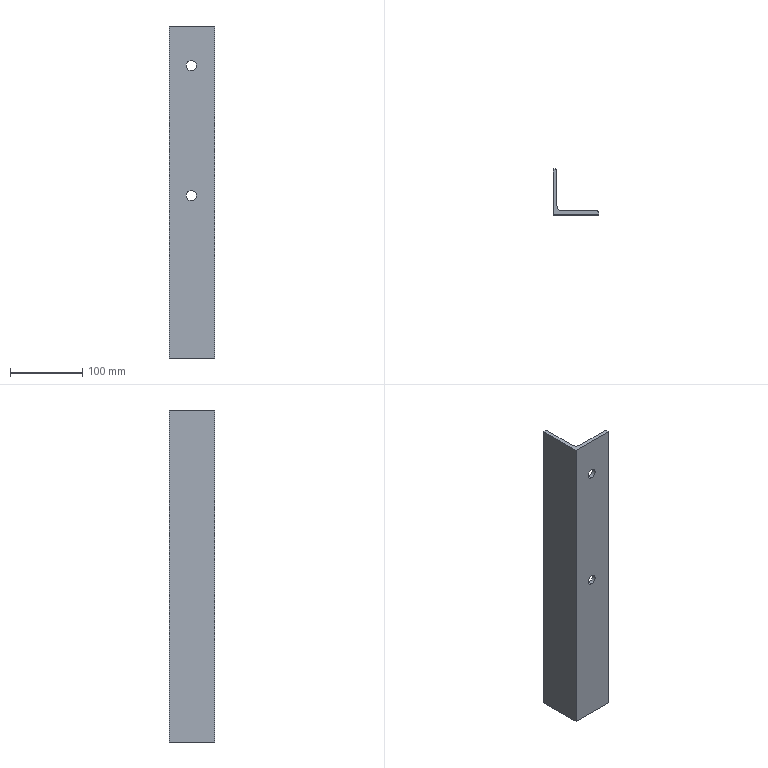Part | NX | features BREP 1 | 1 solid | 15 faces | box 63 x 63 x 460 mm | volume 280553 mm3 | plane 8 | cylinder 7 | commonest cylinder face diameters 14 x5 4.6 x2
STEP:
#1=CARTESIAN_POINT('',(30.5,5.,412.));
#2=VERTEX_POINT('',#1);
#3=CARTESIAN_POINT('',(30.5,5.,398.));
#4=VERTEX_POINT('',#3);
#5=CARTESIAN_POINT('',(30.5,5.,405.));
#6=DIRECTION('',(0.,-1.,0.));
#7=DIRECTION('',(0.,0.,-1.));
#8=AXIS2_PLACEMENT_3D('',#5,#6,#7);
#9=CIRCLE('',#8,7.);
#10=EDGE_CURVE('',#2,#4,#9,.T.);
#11=ORIENTED_EDGE('',*,*,#10,.F.);
#12=CARTESIAN_POINT('',(30.5,0.,412.));
#13=VERTEX_POINT('',#12);
#14=CARTESIAN_POINT('',(30.5,63.,412.));
#15=DIRECTION('',(0.,-1.,0.));
#16=VECTOR('',#15,1000.);
#17=LINE('',#14,#16);
#18=EDGE_CURVE('',#13,#2,#17,.F.);
#19=ORIENTED_EDGE('',*,*,#18,.F.);
#20=CARTESIAN_POINT('',(30.5,0.,398.));
#21=VERTEX_POINT('',#20);
#22=CARTESIAN_POINT('',(30.5,0.,405.));
#23=DIRECTION('',(0.,-1.,0.));
#24=DIRECTION('',(0.,0.,-1.));
#25=AXIS2_PLACEMENT_3D('',#22,#23,#24);
#26=CIRCLE('',#25,7.);
#27=EDGE_CURVE('',#13,#21,#26,.T.);
#28=ORIENTED_EDGE('',*,*,#27,.T.);
#29=CARTESIAN_POINT('',(30.5,63.,398.));
#30=DIRECTION('',(0.,-1.,0.));
#31=VECTOR('',#30,1000.);
#32=LINE('',#29,#31);
#33=EDGE_CURVE('',#21,#4,#32,.F.);
#34=ORIENTED_EDGE('',*,*,#33,.T.);
#35=EDGE_LOOP('',(#11,#19,#28,#34));
#36=FACE_BOUND('',#35,.T.);
#37=CARTESIAN_POINT('',(30.5,63.,405.));
#38=DIRECTION('',(0.,-1.,0.));
#39=DIRECTION('',(0.,0.,1.));
#40=AXIS2_PLACEMENT_3D('',#37,#38,#39);
#41=CYLINDRICAL_SURFACE('',#40,7.);
#42=ADVANCED_FACE('',(#36),#41,.F.);
#43=CARTESIAN_POINT('',(30.5,5.,232.));
#44=VERTEX_POINT('',#43);
#45=CARTESIAN_POINT('',(30.5,5.,218.));
#46=VERTEX_POINT('',#45);
#47=CARTESIAN_POINT('',(30.5,5.,225.));
#48=DIRECTION('',(0.,-1.,0.));
#49=DIRECTION('',(0.,0.,-1.));
#50=AXIS2_PLACEMENT_3D('',#47,#48,#49);
#51=CIRCLE('',#50,7.);
#52=EDGE_CURVE('',#44,#46,#51,.T.);
#53=ORIENTED_EDGE('',*,*,#52,.F.);
#54=CARTESIAN_POINT('',(30.5,0.,232.));
#55=VERTEX_POINT('',#54);
#56=CARTESIAN_POINT('',(30.5,63.,232.));
#57=DIRECTION('',(0.,-1.,0.));
#58=VECTOR('',#57,1000.);
#59=LINE('',#56,#58);
#60=EDGE_CURVE('',#55,#44,#59,.F.);
#61=ORIENTED_EDGE('',*,*,#60,.F.);
#62=CARTESIAN_POINT('',(30.5,0.,218.));
#63=VERTEX_POINT('',#62);
#64=CARTESIAN_POINT('',(30.5,0.,225.));
#65=DIRECTION('',(0.,-1.,0.));
#66=DIRECTION('',(0.,0.,-1.));
#67=AXIS2_PLACEMENT_3D('',#64,#65,#66);
#68=CIRCLE('',#67,7.);
#69=EDGE_CURVE('',#55,#63,#68,.T.);
#70=ORIENTED_EDGE('',*,*,#69,.T.);
#71=CARTESIAN_POINT('',(30.5,63.,218.));
#72=DIRECTION('',(0.,-1.,0.));
#73=VECTOR('',#72,1000.);
#74=LINE('',#71,#73);
#75=EDGE_CURVE('',#63,#46,#74,.F.);
#76=ORIENTED_EDGE('',*,*,#75,.T.);
#77=EDGE_LOOP('',(#53,#61,#70,#76));
#78=FACE_BOUND('',#77,.T.);
#79=CARTESIAN_POINT('',(30.5,63.,225.));
#80=DIRECTION('',(0.,-1.,0.));
#81=DIRECTION('',(0.,0.,1.));
#82=AXIS2_PLACEMENT_3D('',#79,#80,#81);
#83=CYLINDRICAL_SURFACE('',#82,7.);
#84=ADVANCED_FACE('',(#78),#83,.F.);
#85=CARTESIAN_POINT('',(63.,0.,0.));
#86=VERTEX_POINT('',#85);
#87=CARTESIAN_POINT('',(63.,2.7,0.));
#88=VERTEX_POINT('',#87);
#89=CARTESIAN_POINT('',(63.,2.7,0.));
#90=DIRECTION('',(0.,1.,0.));
#91=VECTOR('',#90,1000.);
#92=LINE('',#89,#91);
#93=EDGE_CURVE('',#86,#88,#92,.T.);
#94=ORIENTED_EDGE('',*,*,#93,.T.);
#95=CARTESIAN_POINT('',(63.,2.7,460.));
#96=VERTEX_POINT('',#95);
#97=CARTESIAN_POINT('',(63.,2.7,460.));
#98=DIRECTION('',(0.,0.,-1.));
#99=VECTOR('',#98,1000.);
#100=LINE('',#97,#99);
#101=EDGE_CURVE('',#96,#88,#100,.T.);
#102=ORIENTED_EDGE('',*,*,#101,.F.);
#103=CARTESIAN_POINT('',(63.,0.,460.));
#104=VERTEX_POINT('',#103);
#105=CARTESIAN_POINT('',(63.,2.7,460.));
#106=DIRECTION('',(0.,1.,0.));
#107=VECTOR('',#106,1000.);
#108=LINE('',#105,#107);
#109=EDGE_CURVE('',#104,#96,#108,.T.);
#110=ORIENTED_EDGE('',*,*,#109,.F.);
#111=CARTESIAN_POINT('',(63.,0.,460.));
#112=DIRECTION('',(0.,0.,-1.));
#113=VECTOR('',#112,1000.);
#114=LINE('',#111,#113);
#115=EDGE_CURVE('',#104,#86,#114,.T.);
#116=ORIENTED_EDGE('',*,*,#115,.T.);
#117=EDGE_LOOP('',(#94,#102,#110,#116));
#118=FACE_BOUND('',#117,.T.);
#119=CARTESIAN_POINT('',(63.,2.7,460.));
#120=DIRECTION('',(-1.,0.,0.));
#121=DIRECTION('',(0.,0.,-1.));
#122=AXIS2_PLACEMENT_3D('',#119,#120,#121);
#123=PLANE('',#122);
#124=ADVANCED_FACE('',(#118),#123,.F.);
#125=CARTESIAN_POINT('',(60.7,5.,0.));
#126=VERTEX_POINT('',#125);
#127=CARTESIAN_POINT('',(60.7,2.7,0.));
#128=DIRECTION('',(0.,0.,1.));
#129=DIRECTION('',(1.,0.,0.));
#130=AXIS2_PLACEMENT_3D('',#127,#128,#129);
#131=CIRCLE('',#130,2.3);
#132=EDGE_CURVE('',#88,#126,#131,.T.);
#133=ORIENTED_EDGE('',*,*,#132,.T.);
#134=CARTESIAN_POINT('',(60.7,5.,460.));
#135=VERTEX_POINT('',#134);
#136=CARTESIAN_POINT('',(60.7,5.,460.));
#137=DIRECTION('',(0.,0.,-1.));
#138=VECTOR('',#137,1000.);
#139=LINE('',#136,#138);
#140=EDGE_CURVE('',#135,#126,#139,.T.);
#141=ORIENTED_EDGE('',*,*,#140,.F.);
#142=CARTESIAN_POINT('',(60.7,2.7,460.));
#143=DIRECTION('',(0.,0.,1.));
#144=DIRECTION('',(1.,0.,0.));
#145=AXIS2_PLACEMENT_3D('',#142,#143,#144);
#146=CIRCLE('',#145,2.3);
#147=EDGE_CURVE('',#96,#135,#146,.T.);
#148=ORIENTED_EDGE('',*,*,#147,.F.);
#149=ORIENTED_EDGE('',*,*,#101,.T.);
#150=EDGE_LOOP('',(#133,#141,#148,#149));
#151=FACE_BOUND('',#150,.T.);
#152=CARTESIAN_POINT('',(60.7,2.7,460.));
#153=DIRECTION('',(0.,0.,-1.));
#154=DIRECTION('',(1.,0.,0.));
#155=AXIS2_PLACEMENT_3D('',#152,#153,#154);
#156=CYLINDRICAL_SURFACE('',#155,2.3);
#157=ADVANCED_FACE('',(#151),#156,.T.);
#158=CARTESIAN_POINT('',(30.5,5.,405.));
#159=DIRECTION('',(0.,-1.,0.));
#160=DIRECTION('',(0.,0.,-1.));
#161=AXIS2_PLACEMENT_3D('',#158,#159,#160);
#162=CIRCLE('',#161,7.);
#163=EDGE_CURVE('',#4,#2,#162,.T.);
#164=ORIENTED_EDGE('',*,*,#163,.T.);
#165=ORIENTED_EDGE('',*,*,#10,.T.);
#166=EDGE_LOOP('',(#164,#165));
#167=FACE_BOUND('',#166,.T.);
#168=CARTESIAN_POINT('',(30.5,5.,225.));
#169=DIRECTION('',(0.,-1.,0.));
#170=DIRECTION('',(0.,0.,-1.));
#171=AXIS2_PLACEMENT_3D('',#168,#169,#170);
#172=CIRCLE('',#171,7.);
#173=EDGE_CURVE('',#46,#44,#172,.T.);
#174=ORIENTED_EDGE('',*,*,#173,.T.);
#175=ORIENTED_EDGE('',*,*,#52,.T.);
#176=EDGE_LOOP('',(#174,#175));
#177=FACE_BOUND('',#176,.T.);
#178=CARTESIAN_POINT('',(12.,5.,0.));
#179=VERTEX_POINT('',#178);
#180=CARTESIAN_POINT('',(12.,5.,0.));
#181=DIRECTION('',(-1.,0.,0.));
#182=VECTOR('',#181,1000.);
#183=LINE('',#180,#182);
#184=EDGE_CURVE('',#126,#179,#183,.T.);
#185=ORIENTED_EDGE('',*,*,#184,.T.);
#186=CARTESIAN_POINT('',(12.,5.,460.));
#187=VERTEX_POINT('',#186);
#188=CARTESIAN_POINT('',(12.,5.,460.));
#189=DIRECTION('',(0.,0.,-1.));
#190=VECTOR('',#189,1000.);
#191=LINE('',#188,#190);
#192=EDGE_CURVE('',#187,#179,#191,.T.);
#193=ORIENTED_EDGE('',*,*,#192,.F.);
#194=CARTESIAN_POINT('',(12.,5.,460.));
#195=DIRECTION('',(-1.,0.,0.));
#196=VECTOR('',#195,1000.);
#197=LINE('',#194,#196);
#198=EDGE_CURVE('',#135,#187,#197,.T.);
#199=ORIENTED_EDGE('',*,*,#198,.F.);
#200=ORIENTED_EDGE('',*,*,#140,.T.);
#201=EDGE_LOOP('',(#185,#193,#199,#200));
#202=FACE_BOUND('',#201,.T.);
#203=CARTESIAN_POINT('',(12.,5.,460.));
#204=DIRECTION('',(0.,-1.,0.));
#205=DIRECTION('',(0.,0.,1.));
#206=AXIS2_PLACEMENT_3D('',#203,#204,#205);
#207=PLANE('',#206);
#208=ADVANCED_FACE('',(#167,#177,#202),#207,.F.);
#209=CARTESIAN_POINT('',(5.,12.,0.));
#210=VERTEX_POINT('',#209);
#211=CARTESIAN_POINT('',(12.,12.,0.));
#212=DIRECTION('',(0.,0.,-1.));
#213=DIRECTION('',(1.,0.,0.));
#214=AXIS2_PLACEMENT_3D('',#211,#212,#213);
#215=CIRCLE('',#214,7.);
#216=EDGE_CURVE('',#179,#210,#215,.T.);
#217=ORIENTED_EDGE('',*,*,#216,.T.);
#218=CARTESIAN_POINT('',(5.,12.,460.));
#219=VERTEX_POINT('',#218);
#220=CARTESIAN_POINT('',(5.,12.,460.));
#221=DIRECTION('',(0.,0.,-1.));
#222=VECTOR('',#221,1000.);
#223=LINE('',#220,#222);
#224=EDGE_CURVE('',#219,#210,#223,.T.);
#225=ORIENTED_EDGE('',*,*,#224,.F.);
#226=CARTESIAN_POINT('',(12.,12.,460.));
#227=DIRECTION('',(0.,0.,-1.));
#228=DIRECTION('',(1.,0.,0.));
#229=AXIS2_PLACEMENT_3D('',#226,#227,#228);
#230=CIRCLE('',#229,7.);
#231=EDGE_CURVE('',#187,#219,#230,.T.);
#232=ORIENTED_EDGE('',*,*,#231,.F.);
#233=ORIENTED_EDGE('',*,*,#192,.T.);
#234=EDGE_LOOP('',(#217,#225,#232,#233));
#235=FACE_BOUND('',#234,.T.);
#236=CARTESIAN_POINT('',(12.,12.,460.));
#237=DIRECTION('',(0.,0.,-1.));
#238=DIRECTION('',(1.,0.,0.));
#239=AXIS2_PLACEMENT_3D('',#236,#237,#238);
#240=CYLINDRICAL_SURFACE('',#239,7.);
#241=ADVANCED_FACE('',(#235),#240,.F.);
#242=CARTESIAN_POINT('',(5.,60.7,0.));
#243=VERTEX_POINT('',#242);
#244=CARTESIAN_POINT('',(5.,60.7,0.));
#245=DIRECTION('',(0.,1.,0.));
#246=VECTOR('',#245,1000.);
#247=LINE('',#244,#246);
#248=EDGE_CURVE('',#210,#243,#247,.T.);
#249=ORIENTED_EDGE('',*,*,#248,.T.);
#250=CARTESIAN_POINT('',(5.,60.7,460.));
#251=VERTEX_POINT('',#250);
#252=CARTESIAN_POINT('',(5.,60.7,460.));
#253=DIRECTION('',(0.,0.,-1.));
#254=VECTOR('',#253,1000.);
#255=LINE('',#252,#254);
#256=EDGE_CURVE('',#251,#243,#255,.T.);
#257=ORIENTED_EDGE('',*,*,#256,.F.);
#258=CARTESIAN_POINT('',(5.,60.7,460.));
#259=DIRECTION('',(0.,1.,0.));
#260=VECTOR('',#259,1000.);
#261=LINE('',#258,#260);
#262=EDGE_CURVE('',#219,#251,#261,.T.);
#263=ORIENTED_EDGE('',*,*,#262,.F.);
#264=ORIENTED_EDGE('',*,*,#224,.T.);
#265=EDGE_LOOP('',(#249,#257,#263,#264));
#266=FACE_BOUND('',#265,.T.);
#267=CARTESIAN_POINT('',(5.,60.7,460.));
#268=DIRECTION('',(-1.,0.,0.));
#269=DIRECTION('',(0.,0.,-1.));
#270=AXIS2_PLACEMENT_3D('',#267,#268,#269);
#271=PLANE('',#270);
#272=ADVANCED_FACE('',(#266),#271,.F.);
#273=CARTESIAN_POINT('',(2.7,63.,0.));
#274=VERTEX_POINT('',#273);
#275=CARTESIAN_POINT('',(2.7,60.7,0.));
#276=DIRECTION('',(0.,0.,1.));
#277=DIRECTION('',(1.,0.,0.));
#278=AXIS2_PLACEMENT_3D('',#275,#276,#277);
#279=CIRCLE('',#278,2.3);
#280=EDGE_CURVE('',#243,#274,#279,.T.);
#281=ORIENTED_EDGE('',*,*,#280,.T.);
#282=CARTESIAN_POINT('',(2.7,63.,460.));
#283=VERTEX_POINT('',#282);
#284=CARTESIAN_POINT('',(2.7,63.,460.));
#285=DIRECTION('',(0.,0.,-1.));
#286=VECTOR('',#285,1000.);
#287=LINE('',#284,#286);
#288=EDGE_CURVE('',#283,#274,#287,.T.);
#289=ORIENTED_EDGE('',*,*,#288,.F.);
#290=CARTESIAN_POINT('',(2.7,60.7,460.));
#291=DIRECTION('',(0.,0.,1.));
#292=DIRECTION('',(1.,0.,0.));
#293=AXIS2_PLACEMENT_3D('',#290,#291,#292);
#294=CIRCLE('',#293,2.3);
#295=EDGE_CURVE('',#251,#283,#294,.T.);
#296=ORIENTED_EDGE('',*,*,#295,.F.);
#297=ORIENTED_EDGE('',*,*,#256,.T.);
#298=EDGE_LOOP('',(#281,#289,#296,#297));
#299=FACE_BOUND('',#298,.T.);
#300=CARTESIAN_POINT('',(2.7,60.7,460.));
#301=DIRECTION('',(0.,0.,-1.));
#302=DIRECTION('',(1.,0.,0.));
#303=AXIS2_PLACEMENT_3D('',#300,#301,#302);
#304=CYLINDRICAL_SURFACE('',#303,2.3);
#305=ADVANCED_FACE('',(#299),#304,.T.);
#306=CARTESIAN_POINT('',(0.,63.,0.));
#307=VERTEX_POINT('',#306);
#308=CARTESIAN_POINT('',(0.,63.,0.));
#309=DIRECTION('',(-1.,0.,0.));
#310=VECTOR('',#309,1000.);
#311=LINE('',#308,#310);
#312=EDGE_CURVE('',#274,#307,#311,.T.);
#313=ORIENTED_EDGE('',*,*,#312,.T.);
#314=CARTESIAN_POINT('',(0.,63.,460.));
#315=VERTEX_POINT('',#314);
#316=CARTESIAN_POINT('',(0.,63.,460.));
#317=DIRECTION('',(0.,0.,-1.));
#318=VECTOR('',#317,1000.);
#319=LINE('',#316,#318);
#320=EDGE_CURVE('',#315,#307,#319,.T.);
#321=ORIENTED_EDGE('',*,*,#320,.F.);
#322=CARTESIAN_POINT('',(0.,63.,460.));
#323=DIRECTION('',(-1.,0.,0.));
#324=VECTOR('',#323,1000.);
#325=LINE('',#322,#324);
#326=EDGE_CURVE('',#283,#315,#325,.T.);
#327=ORIENTED_EDGE('',*,*,#326,.F.);
#328=ORIENTED_EDGE('',*,*,#288,.T.);
#329=EDGE_LOOP('',(#313,#321,#327,#328));
#330=FACE_BOUND('',#329,.T.);
#331=CARTESIAN_POINT('',(0.,63.,460.));
#332=DIRECTION('',(0.,-1.,0.));
#333=DIRECTION('',(0.,0.,1.));
#334=AXIS2_PLACEMENT_3D('',#331,#332,#333);
#335=PLANE('',#334);
#336=ADVANCED_FACE('',(#330),#335,.F.);
#337=CARTESIAN_POINT('',(0.,0.,0.));
#338=VERTEX_POINT('',#337);
#339=CARTESIAN_POINT('',(0.,0.,0.));
#340=DIRECTION('',(0.,-1.,0.));
#341=VECTOR('',#340,1000.);
#342=LINE('',#339,#341);
#343=EDGE_CURVE('',#307,#338,#342,.T.);
#344=ORIENTED_EDGE('',*,*,#343,.T.);
#345=CARTESIAN_POINT('',(0.,0.,460.));
#346=VERTEX_POINT('',#345);
#347=CARTESIAN_POINT('',(0.,0.,460.));
#348=DIRECTION('',(0.,0.,-1.));
#349=VECTOR('',#348,1000.);
#350=LINE('',#347,#349);
#351=EDGE_CURVE('',#346,#338,#350,.T.);
#352=ORIENTED_EDGE('',*,*,#351,.F.);
#353=CARTESIAN_POINT('',(0.,0.,460.));
#354=DIRECTION('',(0.,-1.,0.));
#355=VECTOR('',#354,1000.);
#356=LINE('',#353,#355);
#357=EDGE_CURVE('',#315,#346,#356,.T.);
#358=ORIENTED_EDGE('',*,*,#357,.F.);
#359=ORIENTED_EDGE('',*,*,#320,.T.);
#360=EDGE_LOOP('',(#344,#352,#358,#359));
#361=FACE_BOUND('',#360,.T.);
#362=CARTESIAN_POINT('',(0.,0.,460.));
#363=DIRECTION('',(1.,0.,0.));
#364=DIRECTION('',(0.,0.,1.));
#365=AXIS2_PLACEMENT_3D('',#362,#363,#364);
#366=PLANE('',#365);
#367=ADVANCED_FACE('',(#361),#366,.F.);
#368=CARTESIAN_POINT('',(30.5,0.,405.));
#369=DIRECTION('',(0.,-1.,0.));
#370=DIRECTION('',(0.,0.,-1.));
#371=AXIS2_PLACEMENT_3D('',#368,#369,#370);
#372=CIRCLE('',#371,7.);
#373=EDGE_CURVE('',#21,#13,#372,.T.);
#374=ORIENTED_EDGE('',*,*,#373,.F.);
#375=ORIENTED_EDGE('',*,*,#27,.F.);
#376=EDGE_LOOP('',(#374,#375));
#377=FACE_BOUND('',#376,.T.);
#378=CARTESIAN_POINT('',(30.5,0.,225.));
#379=DIRECTION('',(0.,-1.,0.));
#380=DIRECTION('',(0.,0.,-1.));
#381=AXIS2_PLACEMENT_3D('',#378,#379,#380);
#382=CIRCLE('',#381,7.);
#383=EDGE_CURVE('',#63,#55,#382,.T.);
#384=ORIENTED_EDGE('',*,*,#383,.F.);
#385=ORIENTED_EDGE('',*,*,#69,.F.);
#386=EDGE_LOOP('',(#384,#385));
#387=FACE_BOUND('',#386,.T.);
#388=CARTESIAN_POINT('',(63.,0.,0.));
#389=DIRECTION('',(1.,0.,0.));
#390=VECTOR('',#389,1000.);
#391=LINE('',#388,#390);
#392=EDGE_CURVE('',#338,#86,#391,.T.);
#393=ORIENTED_EDGE('',*,*,#392,.T.);
#394=ORIENTED_EDGE('',*,*,#115,.F.);
#395=CARTESIAN_POINT('',(63.,0.,460.));
#396=DIRECTION('',(1.,0.,0.));
#397=VECTOR('',#396,1000.);
#398=LINE('',#395,#397);
#399=EDGE_CURVE('',#346,#104,#398,.T.);
#400=ORIENTED_EDGE('',*,*,#399,.F.);
#401=ORIENTED_EDGE('',*,*,#351,.T.);
#402=EDGE_LOOP('',(#393,#394,#400,#401));
#403=FACE_BOUND('',#402,.T.);
#404=CARTESIAN_POINT('',(63.,0.,460.));
#405=DIRECTION('',(0.,1.,0.));
#406=DIRECTION('',(0.,0.,-1.));
#407=AXIS2_PLACEMENT_3D('',#404,#405,#406);
#408=PLANE('',#407);
#409=ADVANCED_FACE('',(#377,#387,#403),#408,.F.);
#410=ORIENTED_EDGE('',*,*,#109,.T.);
#411=ORIENTED_EDGE('',*,*,#147,.T.);
#412=ORIENTED_EDGE('',*,*,#198,.T.);
#413=ORIENTED_EDGE('',*,*,#231,.T.);
#414=ORIENTED_EDGE('',*,*,#262,.T.);
#415=ORIENTED_EDGE('',*,*,#295,.T.);
#416=ORIENTED_EDGE('',*,*,#326,.T.);
#417=ORIENTED_EDGE('',*,*,#357,.T.);
#418=ORIENTED_EDGE('',*,*,#399,.T.);
#419=EDGE_LOOP('',(#410,#411,#412,#413,#414,#415,#416,#417,#418));
#420=FACE_BOUND('',#419,.T.);
#421=CARTESIAN_POINT('',(2.7,60.7,460.));
#422=DIRECTION('',(0.,0.,1.));
#423=DIRECTION('',(-1.,0.,0.));
#424=AXIS2_PLACEMENT_3D('',#421,#422,#423);
#425=PLANE('',#424);
#426=ADVANCED_FACE('',(#420),#425,.T.);
#427=ORIENTED_EDGE('',*,*,#93,.F.);
#428=ORIENTED_EDGE('',*,*,#392,.F.);
#429=ORIENTED_EDGE('',*,*,#343,.F.);
#430=ORIENTED_EDGE('',*,*,#312,.F.);
#431=ORIENTED_EDGE('',*,*,#280,.F.);
#432=ORIENTED_EDGE('',*,*,#248,.F.);
#433=ORIENTED_EDGE('',*,*,#216,.F.);
#434=ORIENTED_EDGE('',*,*,#184,.F.);
#435=ORIENTED_EDGE('',*,*,#132,.F.);
#436=EDGE_LOOP('',(#427,#428,#429,#430,#431,#432,#433,#434,#435));
#437=FACE_BOUND('',#436,.T.);
#438=CARTESIAN_POINT('',(2.7,60.7,0.));
#439=DIRECTION('',(0.,0.,1.));
#440=DIRECTION('',(-1.,0.,0.));
#441=AXIS2_PLACEMENT_3D('',#438,#439,#440);
#442=PLANE('',#441);
#443=ADVANCED_FACE('',(#437),#442,.F.);
#444=ORIENTED_EDGE('',*,*,#60,.T.);
#445=ORIENTED_EDGE('',*,*,#173,.F.);
#446=ORIENTED_EDGE('',*,*,#75,.F.);
#447=ORIENTED_EDGE('',*,*,#383,.T.);
#448=EDGE_LOOP('',(#444,#445,#446,#447));
#449=FACE_BOUND('',#448,.T.);
#450=CARTESIAN_POINT('',(30.5,63.,225.));
#451=DIRECTION('',(0.,-1.,0.));
#452=DIRECTION('',(0.,0.,1.));
#453=AXIS2_PLACEMENT_3D('',#450,#451,#452);
#454=CYLINDRICAL_SURFACE('',#453,7.);
#455=ADVANCED_FACE('',(#449),#454,.F.);
#456=ORIENTED_EDGE('',*,*,#18,.T.);
#457=ORIENTED_EDGE('',*,*,#163,.F.);
#458=ORIENTED_EDGE('',*,*,#33,.F.);
#459=ORIENTED_EDGE('',*,*,#373,.T.);
#460=EDGE_LOOP('',(#456,#457,#458,#459));
#461=FACE_BOUND('',#460,.T.);
#462=CARTESIAN_POINT('',(30.5,63.,405.));
#463=DIRECTION('',(0.,-1.,0.));
#464=DIRECTION('',(0.,0.,1.));
#465=AXIS2_PLACEMENT_3D('',#462,#463,#464);
#466=CYLINDRICAL_SURFACE('',#465,7.);
#467=ADVANCED_FACE('',(#461),#466,.F.);
#468=CLOSED_SHELL('',(#42,#84,#124,#157,#208,#241,#272,#305,#336,#367,#409,#426,#443,#455,#467));
#469=MANIFOLD_SOLID_BREP('',#468);
#470=(LENGTH_UNIT()NAMED_UNIT(*)SI_UNIT(.MILLI.,.METRE.));
#471=UNCERTAINTY_MEASURE_WITH_UNIT(LENGTH_MEASURE(0.00001),#470,'','');
#472=(NAMED_UNIT(*)PLANE_ANGLE_UNIT()SI_UNIT($,.RADIAN.));
#473=(NAMED_UNIT(*)SI_UNIT($,.STERADIAN.)SOLID_ANGLE_UNIT());
#474=(GEOMETRIC_REPRESENTATION_CONTEXT(3)GLOBAL_UNCERTAINTY_ASSIGNED_CONTEXT((#471))GLOBAL_UNIT_ASSIGNED_CONTEXT((#470,#472,#473))REPRESENTATION_CONTEXT('',''));
#475=ADVANCED_BREP_SHAPE_REPRESENTATION('',(#469),#474);